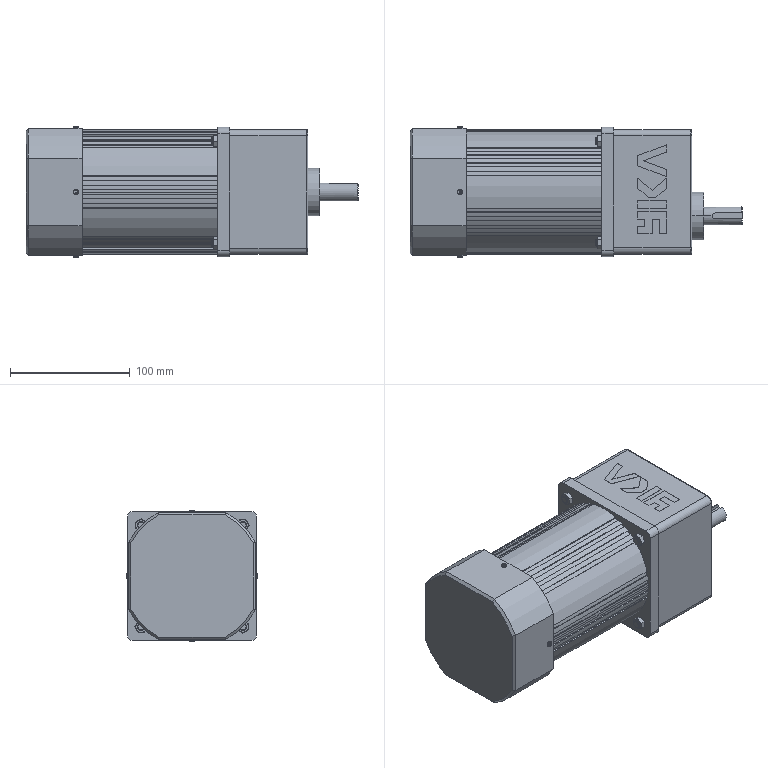Part | STEP file | 2 solids | 366 faces | box 277 x 108.652 x 108.652 mm | volume 2253105 mm3 | plane 198 | cylinder 105 | cone 41 | spline 22 | commonest cylinder face diameters 104 x25 102 x24 4.42 x8 6 x8 9 x8 9.2 x8